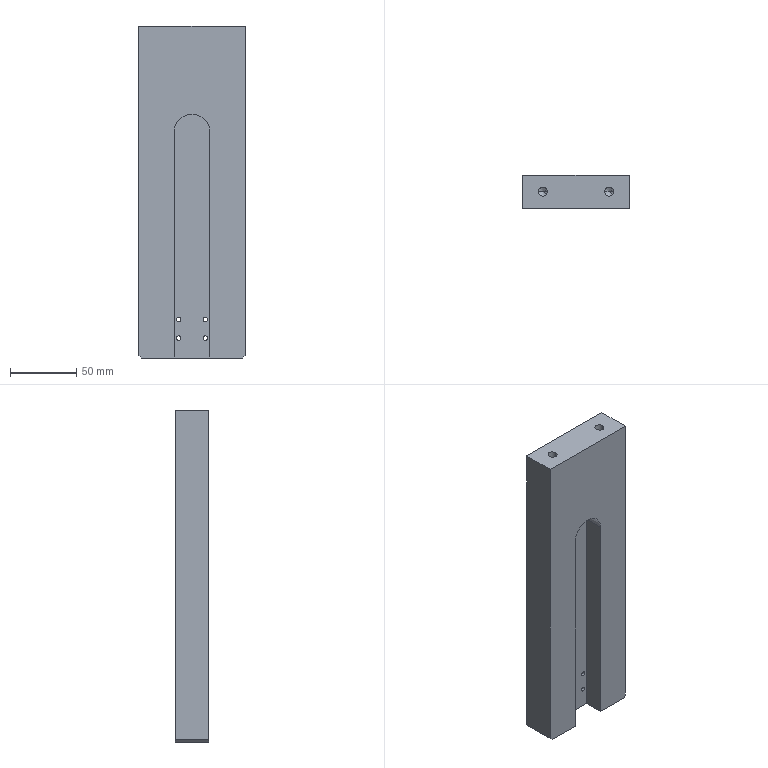Part | SolidWorks | features HoleWzd 5, ICE 2, MirrorPattern 2, Chamfer 1, Extrusion 1 | 1 solid | 28 faces | box 80 x 25 x 250 mm | volume 424930 mm3 | cylinder 13 | plane 11 | cone 4 | commonest cylinder face diameters 3.3 x8 6.8 x4 27 x1
STEP:
#1=CARTESIAN_POINT('',(-28.4,0.,-19.75));
#2=VERTEX_POINT('',#1);
#3=CARTESIAN_POINT('',(-21.6,0.,-19.75));
#4=VERTEX_POINT('',#3);
#5=CARTESIAN_POINT('',(-25.,0.,-19.75));
#6=DIRECTION('',(0.,0.,1.));
#7=DIRECTION('',(1.,0.,0.));
#8=AXIS2_PLACEMENT_3D('',#5,#6,#7);
#9=CIRCLE('',#8,3.4);
#10=EDGE_CURVE('',#2,#4,#9,.T.);
#11=ORIENTED_EDGE('',*,*,#10,.F.);
#12=CARTESIAN_POINT('',(-28.4,0.,0.));
#13=VERTEX_POINT('',#12);
#14=CARTESIAN_POINT('',(-28.4,0.,0.));
#15=DIRECTION('',(0.,0.,1.));
#16=VECTOR('',#15,1000.);
#17=LINE('',#14,#16);
#18=EDGE_CURVE('',#2,#13,#17,.T.);
#19=ORIENTED_EDGE('',*,*,#18,.T.);
#20=CARTESIAN_POINT('',(-21.6,0.,0.));
#21=VERTEX_POINT('',#20);
#22=CARTESIAN_POINT('',(-25.,0.,0.));
#23=DIRECTION('',(0.,0.,1.));
#24=DIRECTION('',(1.,0.,0.));
#25=AXIS2_PLACEMENT_3D('',#22,#23,#24);
#26=CIRCLE('',#25,3.4);
#27=EDGE_CURVE('',#13,#21,#26,.T.);
#28=ORIENTED_EDGE('',*,*,#27,.T.);
#29=CARTESIAN_POINT('',(-21.6,0.,0.));
#30=DIRECTION('',(0.,0.,1.));
#31=VECTOR('',#30,1000.);
#32=LINE('',#29,#31);
#33=EDGE_CURVE('',#4,#21,#32,.T.);
#34=ORIENTED_EDGE('',*,*,#33,.F.);
#35=EDGE_LOOP('',(#11,#19,#28,#34));
#36=FACE_OUTER_BOUND('',#35,.T.);
#37=CARTESIAN_POINT('',(-25.,0.,0.));
#38=DIRECTION('',(0.,0.,1.));
#39=DIRECTION('',(1.,0.,0.));
#40=AXIS2_PLACEMENT_3D('',#37,#38,#39);
#41=CYLINDRICAL_SURFACE('',#40,3.4);
#42=ADVANCED_FACE('',(#36),#41,.F.);
#43=CARTESIAN_POINT('',(-25.,0.,-21.793));
#44=VERTEX_POINT('',#43);
#45=CARTESIAN_POINT('',(-21.6,0.,-19.75));
#46=DIRECTION('',(0.8572,0.,0.515));
#47=VECTOR('',#46,1000.);
#48=LINE('',#45,#47);
#49=EDGE_CURVE('',#44,#4,#48,.T.);
#50=ORIENTED_EDGE('',*,*,#49,.F.);
#51=CARTESIAN_POINT('',(-28.4,0.,-19.75));
#52=DIRECTION('',(-0.8572,0.,0.515));
#53=VECTOR('',#52,1000.);
#54=LINE('',#51,#53);
#55=EDGE_CURVE('',#44,#2,#54,.T.);
#56=ORIENTED_EDGE('',*,*,#55,.T.);
#57=ORIENTED_EDGE('',*,*,#10,.T.);
#58=EDGE_LOOP('',(#50,#56,#57));
#59=FACE_OUTER_BOUND('',#58,.T.);
#60=CARTESIAN_POINT('',(-25.,0.,-19.75));
#61=DIRECTION('',(0.,0.,1.));
#62=DIRECTION('',(1.,0.,0.));
#63=AXIS2_PLACEMENT_3D('',#60,#61,#62);
#64=CONICAL_SURFACE('',#63,3.4,1.03);
#65=ADVANCED_FACE('',(#59),#64,.F.);
#66=CARTESIAN_POINT('',(21.6,0.,-19.75));
#67=VERTEX_POINT('',#66);
#68=CARTESIAN_POINT('',(28.4,0.,-19.75));
#69=VERTEX_POINT('',#68);
#70=CARTESIAN_POINT('',(25.,0.,-19.75));
#71=DIRECTION('',(0.,0.,1.));
#72=DIRECTION('',(1.,0.,0.));
#73=AXIS2_PLACEMENT_3D('',#70,#71,#72);
#74=CIRCLE('',#73,3.4);
#75=EDGE_CURVE('',#67,#69,#74,.T.);
#76=ORIENTED_EDGE('',*,*,#75,.F.);
#77=CARTESIAN_POINT('',(21.6,0.,0.));
#78=VERTEX_POINT('',#77);
#79=CARTESIAN_POINT('',(21.6,0.,0.));
#80=DIRECTION('',(0.,0.,1.));
#81=VECTOR('',#80,1000.);
#82=LINE('',#79,#81);
#83=EDGE_CURVE('',#67,#78,#82,.T.);
#84=ORIENTED_EDGE('',*,*,#83,.T.);
#85=CARTESIAN_POINT('',(28.4,0.,0.));
#86=VERTEX_POINT('',#85);
#87=CARTESIAN_POINT('',(25.,0.,0.));
#88=DIRECTION('',(0.,0.,1.));
#89=DIRECTION('',(1.,0.,0.));
#90=AXIS2_PLACEMENT_3D('',#87,#88,#89);
#91=CIRCLE('',#90,3.4);
#92=EDGE_CURVE('',#78,#86,#91,.T.);
#93=ORIENTED_EDGE('',*,*,#92,.T.);
#94=CARTESIAN_POINT('',(28.4,0.,0.));
#95=DIRECTION('',(0.,0.,1.));
#96=VECTOR('',#95,1000.);
#97=LINE('',#94,#96);
#98=EDGE_CURVE('',#69,#86,#97,.T.);
#99=ORIENTED_EDGE('',*,*,#98,.F.);
#100=EDGE_LOOP('',(#76,#84,#93,#99));
#101=FACE_OUTER_BOUND('',#100,.T.);
#102=CARTESIAN_POINT('',(25.,0.,0.));
#103=DIRECTION('',(0.,0.,1.));
#104=DIRECTION('',(1.,0.,0.));
#105=AXIS2_PLACEMENT_3D('',#102,#103,#104);
#106=CYLINDRICAL_SURFACE('',#105,3.4);
#107=ADVANCED_FACE('',(#101),#106,.F.);
#108=CARTESIAN_POINT('',(25.,0.,-21.793));
#109=VERTEX_POINT('',#108);
#110=CARTESIAN_POINT('',(28.4,0.,-19.75));
#111=DIRECTION('',(0.8572,0.,0.515));
#112=VECTOR('',#111,1000.);
#113=LINE('',#110,#112);
#114=EDGE_CURVE('',#109,#69,#113,.T.);
#115=ORIENTED_EDGE('',*,*,#114,.F.);
#116=CARTESIAN_POINT('',(21.6,0.,-19.75));
#117=DIRECTION('',(-0.8572,0.,0.515));
#118=VECTOR('',#117,1000.);
#119=LINE('',#116,#118);
#120=EDGE_CURVE('',#109,#67,#119,.T.);
#121=ORIENTED_EDGE('',*,*,#120,.T.);
#122=ORIENTED_EDGE('',*,*,#75,.T.);
#123=EDGE_LOOP('',(#115,#121,#122));
#124=FACE_OUTER_BOUND('',#123,.T.);
#125=CARTESIAN_POINT('',(25.,0.,-19.75));
#126=DIRECTION('',(0.,0.,1.));
#127=DIRECTION('',(1.,0.,0.));
#128=AXIS2_PLACEMENT_3D('',#125,#126,#127);
#129=CONICAL_SURFACE('',#128,3.4,1.03);
#130=ADVANCED_FACE('',(#124),#129,.F.);
#131=CARTESIAN_POINT('',(-10.,2.5,-233.35));
#132=VERTEX_POINT('',#131);
#133=CARTESIAN_POINT('',(-10.,2.5,-236.65));
#134=VERTEX_POINT('',#133);
#135=CARTESIAN_POINT('',(-10.,2.5,-235.));
#136=DIRECTION('',(0.,-1.,0.));
#137=DIRECTION('',(0.,0.,-1.));
#138=AXIS2_PLACEMENT_3D('',#135,#136,#137);
#139=CIRCLE('',#138,1.65);
#140=EDGE_CURVE('',#132,#134,#139,.T.);
#141=ORIENTED_EDGE('',*,*,#140,.T.);
#142=CARTESIAN_POINT('',(-10.,12.5,-236.65));
#143=VERTEX_POINT('',#142);
#144=CARTESIAN_POINT('',(-10.,12.5,-236.65));
#145=DIRECTION('',(0.,1.,0.));
#146=VECTOR('',#145,1000.);
#147=LINE('',#144,#146);
#148=EDGE_CURVE('',#134,#143,#147,.T.);
#149=ORIENTED_EDGE('',*,*,#148,.T.);
#150=CARTESIAN_POINT('',(-10.,12.5,-233.35));
#151=VERTEX_POINT('',#150);
#152=CARTESIAN_POINT('',(-10.,12.5,-235.));
#153=DIRECTION('',(0.,1.,0.));
#154=DIRECTION('',(0.,0.,1.));
#155=AXIS2_PLACEMENT_3D('',#152,#153,#154);
#156=CIRCLE('',#155,1.65);
#157=EDGE_CURVE('',#143,#151,#156,.T.);
#158=ORIENTED_EDGE('',*,*,#157,.T.);
#159=CARTESIAN_POINT('',(-10.,12.5,-233.35));
#160=DIRECTION('',(0.,1.,0.));
#161=VECTOR('',#160,1000.);
#162=LINE('',#159,#161);
#163=EDGE_CURVE('',#132,#151,#162,.T.);
#164=ORIENTED_EDGE('',*,*,#163,.F.);
#165=EDGE_LOOP('',(#141,#149,#158,#164));
#166=FACE_OUTER_BOUND('',#165,.T.);
#167=CARTESIAN_POINT('',(-10.,12.5,-235.));
#168=DIRECTION('',(0.,1.,0.));
#169=DIRECTION('',(0.,0.,1.));
#170=AXIS2_PLACEMENT_3D('',#167,#168,#169);
#171=CYLINDRICAL_SURFACE('',#170,1.65);
#172=ADVANCED_FACE('',(#166),#171,.F.);
#173=CARTESIAN_POINT('',(-10.,2.5,-219.35));
#174=VERTEX_POINT('',#173);
#175=CARTESIAN_POINT('',(-10.,2.5,-222.65));
#176=VERTEX_POINT('',#175);
#177=CARTESIAN_POINT('',(-10.,2.5,-221.));
#178=DIRECTION('',(0.,-1.,0.));
#179=DIRECTION('',(0.,0.,-1.));
#180=AXIS2_PLACEMENT_3D('',#177,#178,#179);
#181=CIRCLE('',#180,1.65);
#182=EDGE_CURVE('',#174,#176,#181,.T.);
#183=ORIENTED_EDGE('',*,*,#182,.T.);
#184=CARTESIAN_POINT('',(-10.,12.5,-222.65));
#185=VERTEX_POINT('',#184);
#186=CARTESIAN_POINT('',(-10.,12.5,-222.65));
#187=DIRECTION('',(0.,1.,0.));
#188=VECTOR('',#187,1000.);
#189=LINE('',#186,#188);
#190=EDGE_CURVE('',#176,#185,#189,.T.);
#191=ORIENTED_EDGE('',*,*,#190,.T.);
#192=CARTESIAN_POINT('',(-10.,12.5,-219.35));
#193=VERTEX_POINT('',#192);
#194=CARTESIAN_POINT('',(-10.,12.5,-221.));
#195=DIRECTION('',(0.,1.,0.));
#196=DIRECTION('',(0.,0.,1.));
#197=AXIS2_PLACEMENT_3D('',#194,#195,#196);
#198=CIRCLE('',#197,1.65);
#199=EDGE_CURVE('',#185,#193,#198,.T.);
#200=ORIENTED_EDGE('',*,*,#199,.T.);
#201=CARTESIAN_POINT('',(-10.,12.5,-219.35));
#202=DIRECTION('',(0.,1.,0.));
#203=VECTOR('',#202,1000.);
#204=LINE('',#201,#203);
#205=EDGE_CURVE('',#174,#193,#204,.T.);
#206=ORIENTED_EDGE('',*,*,#205,.F.);
#207=EDGE_LOOP('',(#183,#191,#200,#206));
#208=FACE_OUTER_BOUND('',#207,.T.);
#209=CARTESIAN_POINT('',(-10.,12.5,-221.));
#210=DIRECTION('',(0.,1.,0.));
#211=DIRECTION('',(0.,0.,1.));
#212=AXIS2_PLACEMENT_3D('',#209,#210,#211);
#213=CYLINDRICAL_SURFACE('',#212,1.65);
#214=ADVANCED_FACE('',(#208),#213,.F.);
#215=CARTESIAN_POINT('',(10.,2.5,-219.35));
#216=VERTEX_POINT('',#215);
#217=CARTESIAN_POINT('',(10.,2.5,-222.65));
#218=VERTEX_POINT('',#217);
#219=CARTESIAN_POINT('',(10.,2.5,-221.));
#220=DIRECTION('',(0.,-1.,0.));
#221=DIRECTION('',(0.,0.,-1.));
#222=AXIS2_PLACEMENT_3D('',#219,#220,#221);
#223=CIRCLE('',#222,1.65);
#224=EDGE_CURVE('',#216,#218,#223,.T.);
#225=ORIENTED_EDGE('',*,*,#224,.T.);
#226=CARTESIAN_POINT('',(10.,12.5,-222.65));
#227=VERTEX_POINT('',#226);
#228=CARTESIAN_POINT('',(10.,12.5,-222.65));
#229=DIRECTION('',(0.,1.,0.));
#230=VECTOR('',#229,1000.);
#231=LINE('',#228,#230);
#232=EDGE_CURVE('',#218,#227,#231,.T.);
#233=ORIENTED_EDGE('',*,*,#232,.T.);
#234=CARTESIAN_POINT('',(10.,12.5,-219.35));
#235=VERTEX_POINT('',#234);
#236=CARTESIAN_POINT('',(10.,12.5,-221.));
#237=DIRECTION('',(0.,1.,0.));
#238=DIRECTION('',(0.,0.,1.));
#239=AXIS2_PLACEMENT_3D('',#236,#237,#238);
#240=CIRCLE('',#239,1.65);
#241=EDGE_CURVE('',#227,#235,#240,.T.);
#242=ORIENTED_EDGE('',*,*,#241,.T.);
#243=CARTESIAN_POINT('',(10.,12.5,-219.35));
#244=DIRECTION('',(0.,1.,0.));
#245=VECTOR('',#244,1000.);
#246=LINE('',#243,#245);
#247=EDGE_CURVE('',#216,#235,#246,.T.);
#248=ORIENTED_EDGE('',*,*,#247,.F.);
#249=EDGE_LOOP('',(#225,#233,#242,#248));
#250=FACE_OUTER_BOUND('',#249,.T.);
#251=CARTESIAN_POINT('',(10.,12.5,-221.));
#252=DIRECTION('',(0.,1.,0.));
#253=DIRECTION('',(0.,0.,1.));
#254=AXIS2_PLACEMENT_3D('',#251,#252,#253);
#255=CYLINDRICAL_SURFACE('',#254,1.65);
#256=ADVANCED_FACE('',(#250),#255,.F.);
#257=CARTESIAN_POINT('',(10.,2.5,-233.35));
#258=VERTEX_POINT('',#257);
#259=CARTESIAN_POINT('',(10.,2.5,-236.65));
#260=VERTEX_POINT('',#259);
#261=CARTESIAN_POINT('',(10.,2.5,-235.));
#262=DIRECTION('',(0.,-1.,0.));
#263=DIRECTION('',(0.,0.,-1.));
#264=AXIS2_PLACEMENT_3D('',#261,#262,#263);
#265=CIRCLE('',#264,1.65);
#266=EDGE_CURVE('',#258,#260,#265,.T.);
#267=ORIENTED_EDGE('',*,*,#266,.T.);
#268=CARTESIAN_POINT('',(10.,12.5,-236.65));
#269=VERTEX_POINT('',#268);
#270=CARTESIAN_POINT('',(10.,12.5,-236.65));
#271=DIRECTION('',(0.,1.,0.));
#272=VECTOR('',#271,1000.);
#273=LINE('',#270,#272);
#274=EDGE_CURVE('',#260,#269,#273,.T.);
#275=ORIENTED_EDGE('',*,*,#274,.T.);
#276=CARTESIAN_POINT('',(10.,12.5,-233.35));
#277=VERTEX_POINT('',#276);
#278=CARTESIAN_POINT('',(10.,12.5,-235.));
#279=DIRECTION('',(0.,1.,0.));
#280=DIRECTION('',(0.,0.,1.));
#281=AXIS2_PLACEMENT_3D('',#278,#279,#280);
#282=CIRCLE('',#281,1.65);
#283=EDGE_CURVE('',#269,#277,#282,.T.);
#284=ORIENTED_EDGE('',*,*,#283,.T.);
#285=CARTESIAN_POINT('',(10.,12.5,-233.35));
#286=DIRECTION('',(0.,1.,0.));
#287=VECTOR('',#286,1000.);
#288=LINE('',#285,#287);
#289=EDGE_CURVE('',#258,#277,#288,.T.);
#290=ORIENTED_EDGE('',*,*,#289,.F.);
#291=EDGE_LOOP('',(#267,#275,#284,#290));
#292=FACE_OUTER_BOUND('',#291,.T.);
#293=CARTESIAN_POINT('',(10.,12.5,-235.));
#294=DIRECTION('',(0.,1.,0.));
#295=DIRECTION('',(0.,0.,1.));
#296=AXIS2_PLACEMENT_3D('',#293,#294,#295);
#297=CYLINDRICAL_SURFACE('',#296,1.65);
#298=ADVANCED_FACE('',(#292),#297,.F.);
#299=CARTESIAN_POINT('',(-25.,0.,0.));
#300=DIRECTION('',(0.,0.,1.));
#301=DIRECTION('',(1.,0.,0.));
#302=AXIS2_PLACEMENT_3D('',#299,#300,#301);
#303=CIRCLE('',#302,3.4);
#304=EDGE_CURVE('',#21,#13,#303,.T.);
#305=ORIENTED_EDGE('',*,*,#304,.F.);
#306=ORIENTED_EDGE('',*,*,#27,.F.);
#307=EDGE_LOOP('',(#305,#306));
#308=FACE_BOUND('',#307,.T.);
#309=CARTESIAN_POINT('',(25.,0.,0.));
#310=DIRECTION('',(0.,0.,1.));
#311=DIRECTION('',(1.,0.,0.));
#312=AXIS2_PLACEMENT_3D('',#309,#310,#311);
#313=CIRCLE('',#312,3.4);
#314=EDGE_CURVE('',#86,#78,#313,.T.);
#315=ORIENTED_EDGE('',*,*,#314,.F.);
#316=ORIENTED_EDGE('',*,*,#92,.F.);
#317=EDGE_LOOP('',(#315,#316));
#318=FACE_BOUND('',#317,.T.);
#319=CARTESIAN_POINT('',(-40.,-12.5,0.));
#320=VERTEX_POINT('',#319);
#321=CARTESIAN_POINT('',(40.,-12.5,0.));
#322=VERTEX_POINT('',#321);
#323=CARTESIAN_POINT('',(-75.,-12.5,0.));
#324=DIRECTION('',(1.,0.,0.));
#325=VECTOR('',#324,1000.);
#326=LINE('',#323,#325);
#327=EDGE_CURVE('',#320,#322,#326,.T.);
#328=ORIENTED_EDGE('',*,*,#327,.T.);
#329=CARTESIAN_POINT('',(40.,12.5,0.));
#330=VERTEX_POINT('',#329);
#331=CARTESIAN_POINT('',(40.,12.5,0.));
#332=DIRECTION('',(0.,1.,0.));
#333=VECTOR('',#332,1000.);
#334=LINE('',#331,#333);
#335=EDGE_CURVE('',#322,#330,#334,.T.);
#336=ORIENTED_EDGE('',*,*,#335,.T.);
#337=CARTESIAN_POINT('',(-40.,12.5,0.));
#338=VERTEX_POINT('',#337);
#339=CARTESIAN_POINT('',(-75.,12.5,0.));
#340=DIRECTION('',(1.,0.,0.));
#341=VECTOR('',#340,1000.);
#342=LINE('',#339,#341);
#343=EDGE_CURVE('',#338,#330,#342,.T.);
#344=ORIENTED_EDGE('',*,*,#343,.F.);
#345=CARTESIAN_POINT('',(-40.,12.5,0.));
#346=DIRECTION('',(0.,-1.,0.));
#347=VECTOR('',#346,1000.);
#348=LINE('',#345,#347);
#349=EDGE_CURVE('',#338,#320,#348,.T.);
#350=ORIENTED_EDGE('',*,*,#349,.T.);
#351=EDGE_LOOP('',(#328,#336,#344,#350));
#352=FACE_OUTER_BOUND('',#351,.T.);
#353=CARTESIAN_POINT('',(-75.,12.5,0.));
#354=DIRECTION('',(0.,0.,-1.));
#355=DIRECTION('',(-1.,0.,0.));
#356=AXIS2_PLACEMENT_3D('',#353,#354,#355);
#357=PLANE('',#356);
#358=ADVANCED_FACE('',(#308,#318,#352),#357,.F.);
#359=CARTESIAN_POINT('',(40.,-12.5,-248.));
#360=VERTEX_POINT('',#359);
#361=CARTESIAN_POINT('',(40.,-12.5,-12.));
#362=DIRECTION('',(0.,0.,-1.));
#363=VECTOR('',#362,1000.);
#364=LINE('',#361,#363);
#365=EDGE_CURVE('',#322,#360,#364,.T.);
#366=ORIENTED_EDGE('',*,*,#365,.T.);
#367=CARTESIAN_POINT('',(40.,12.5,-248.));
#368=VERTEX_POINT('',#367);
#369=CARTESIAN_POINT('',(40.,12.5,-248.));
#370=DIRECTION('',(0.,1.,0.));
#371=VECTOR('',#370,1000.);
#372=LINE('',#369,#371);
#373=EDGE_CURVE('',#360,#368,#372,.T.);
#374=ORIENTED_EDGE('',*,*,#373,.T.);
#375=CARTESIAN_POINT('',(40.,12.5,-12.));
#376=DIRECTION('',(0.,0.,-1.));
#377=VECTOR('',#376,1000.);
#378=LINE('',#375,#377);
#379=EDGE_CURVE('',#330,#368,#378,.T.);
#380=ORIENTED_EDGE('',*,*,#379,.F.);
#381=ORIENTED_EDGE('',*,*,#335,.F.);
#382=EDGE_LOOP('',(#366,#374,#380,#381));
#383=FACE_OUTER_BOUND('',#382,.T.);
#384=CARTESIAN_POINT('',(40.,12.5,-12.));
#385=DIRECTION('',(-1.,0.,0.));
#386=DIRECTION('',(0.,0.,1.));
#387=AXIS2_PLACEMENT_3D('',#384,#385,#386);
#388=PLANE('',#387);
#389=ADVANCED_FACE('',(#383),#388,.F.);
#390=CARTESIAN_POINT('',(38.,-12.5,-250.));
#391=VERTEX_POINT('',#390);
#392=CARTESIAN_POINT('',(13.5,-12.5,-250.));
#393=VERTEX_POINT('',#392);
#394=CARTESIAN_POINT('',(40.,-12.5,-250.));
#395=DIRECTION('',(-1.,0.,0.));
#396=VECTOR('',#395,1000.);
#397=LINE('',#394,#396);
#398=EDGE_CURVE('',#391,#393,#397,.T.);
#399=ORIENTED_EDGE('',*,*,#398,.T.);
#400=CARTESIAN_POINT('',(13.5,2.5,-250.));
#401=VERTEX_POINT('',#400);
#402=CARTESIAN_POINT('',(13.5,2.5,-250.));
#403=DIRECTION('',(0.,-1.,0.));
#404=VECTOR('',#403,1000.);
#405=LINE('',#402,#404);
#406=EDGE_CURVE('',#401,#393,#405,.T.);
#407=ORIENTED_EDGE('',*,*,#406,.F.);
#408=CARTESIAN_POINT('',(-13.5,2.5,-250.));
#409=VERTEX_POINT('',#408);
#410=CARTESIAN_POINT('',(40.,2.5,-250.));
#411=DIRECTION('',(1.,0.,0.));
#412=VECTOR('',#411,1000.);
#413=LINE('',#410,#412);
#414=EDGE_CURVE('',#409,#401,#413,.T.);
#415=ORIENTED_EDGE('',*,*,#414,.F.);
#416=CARTESIAN_POINT('',(-13.5,-12.5,-250.));
#417=VERTEX_POINT('',#416);
#418=CARTESIAN_POINT('',(-13.5,2.5,-250.));
#419=DIRECTION('',(0.,-1.,0.));
#420=VECTOR('',#419,1000.);
#421=LINE('',#418,#420);
#422=EDGE_CURVE('',#409,#417,#421,.T.);
#423=ORIENTED_EDGE('',*,*,#422,.T.);
#424=CARTESIAN_POINT('',(-38.,-12.5,-250.));
#425=VERTEX_POINT('',#424);
#426=CARTESIAN_POINT('',(40.,-12.5,-250.));
#427=DIRECTION('',(-1.,0.,0.));
#428=VECTOR('',#427,1000.);
#429=LINE('',#426,#428);
#430=EDGE_CURVE('',#417,#425,#429,.T.);
#431=ORIENTED_EDGE('',*,*,#430,.T.);
#432=CARTESIAN_POINT('',(-38.,12.5,-250.));
#433=VERTEX_POINT('',#432);
#434=CARTESIAN_POINT('',(-38.,12.5,-250.));
#435=DIRECTION('',(0.,1.,0.));
#436=VECTOR('',#435,1000.);
#437=LINE('',#434,#436);
#438=EDGE_CURVE('',#425,#433,#437,.T.);
#439=ORIENTED_EDGE('',*,*,#438,.T.);
#440=CARTESIAN_POINT('',(38.,12.5,-250.));
#441=VERTEX_POINT('',#440);
#442=CARTESIAN_POINT('',(40.,12.5,-250.));
#443=DIRECTION('',(-1.,0.,0.));
#444=VECTOR('',#443,1000.);
#445=LINE('',#442,#444);
#446=EDGE_CURVE('',#441,#433,#445,.T.);
#447=ORIENTED_EDGE('',*,*,#446,.F.);
#448=CARTESIAN_POINT('',(38.,12.5,-250.));
#449=DIRECTION('',(0.,-1.,0.));
#450=VECTOR('',#449,1000.);
#451=LINE('',#448,#450);
#452=EDGE_CURVE('',#441,#391,#451,.T.);
#453=ORIENTED_EDGE('',*,*,#452,.T.);
#454=EDGE_LOOP('',(#399,#407,#415,#423,#431,#439,#447,#453));
#455=FACE_OUTER_BOUND('',#454,.T.);
#456=CARTESIAN_POINT('',(40.,12.5,-250.));
#457=DIRECTION('',(0.,0.,1.));
#458=DIRECTION('',(1.,0.,0.));
#459=AXIS2_PLACEMENT_3D('',#456,#457,#458);
#460=PLANE('',#459);
#461=ADVANCED_FACE('',(#455),#460,.F.);
#462=CARTESIAN_POINT('',(-40.,12.5,-248.));
#463=VERTEX_POINT('',#462);
#464=CARTESIAN_POINT('',(-40.,12.5,-250.));
#465=DIRECTION('',(0.,0.,1.));
#466=VECTOR('',#465,1000.);
#467=LINE('',#464,#466);
#468=EDGE_CURVE('',#463,#338,#467,.T.);
#469=ORIENTED_EDGE('',*,*,#468,.F.);
#470=CARTESIAN_POINT('',(-40.,-12.5,-248.));
#471=VERTEX_POINT('',#470);
#472=CARTESIAN_POINT('',(-40.,12.5,-248.));
#473=DIRECTION('',(0.,-1.,0.));
#474=VECTOR('',#473,1000.);
#475=LINE('',#472,#474);
#476=EDGE_CURVE('',#463,#471,#475,.T.);
#477=ORIENTED_EDGE('',*,*,#476,.T.);
#478=CARTESIAN_POINT('',(-40.,-12.5,-250.));
#479=DIRECTION('',(0.,0.,1.));
#480=VECTOR('',#479,1000.);
#481=LINE('',#478,#480);
#482=EDGE_CURVE('',#471,#320,#481,.T.);
#483=ORIENTED_EDGE('',*,*,#482,.T.);
#484=ORIENTED_EDGE('',*,*,#349,.F.);
#485=EDGE_LOOP('',(#469,#477,#483,#484));
#486=FACE_OUTER_BOUND('',#485,.T.);
#487=CARTESIAN_POINT('',(-40.,12.5,-250.));
#488=DIRECTION('',(1.,0.,0.));
#489=DIRECTION('',(0.,0.,-1.));
#490=AXIS2_PLACEMENT_3D('',#487,#488,#489);
#491=PLANE('',#490);
#492=ADVANCED_FACE('',(#486),#491,.F.);
#493=ORIENTED_EDGE('',*,*,#343,.T.);
#494=ORIENTED_EDGE('',*,*,#379,.T.);
#495=CARTESIAN_POINT('',(144.,12.5,-144.));
#496=DIRECTION('',(-0.7071,0.,-0.7071));
#497=VECTOR('',#496,1000.);
#498=LINE('',#495,#497);
#499=EDGE_CURVE('',#368,#441,#498,.T.);
#500=ORIENTED_EDGE('',*,*,#499,.T.);
#501=ORIENTED_EDGE('',*,*,#446,.T.);
#502=CARTESIAN_POINT('',(-144.,12.5,-144.));
#503=DIRECTION('',(-0.7071,0.,0.7071));
#504=VECTOR('',#503,1000.);
#505=LINE('',#502,#504);
#506=EDGE_CURVE('',#433,#463,#505,.T.);
#507=ORIENTED_EDGE('',*,*,#506,.T.);
#508=ORIENTED_EDGE('',*,*,#468,.T.);
#509=EDGE_LOOP('',(#493,#494,#500,#501,#507,#508));
#510=FACE_OUTER_BOUND('',#509,.T.);
#511=CARTESIAN_POINT('',(-10.,12.5,-235.));
#512=DIRECTION('',(0.,1.,0.));
#513=DIRECTION('',(0.,0.,1.));
#514=AXIS2_PLACEMENT_3D('',#511,#512,#513);
#515=CIRCLE('',#514,1.65);
#516=EDGE_CURVE('',#151,#143,#515,.T.);
#517=ORIENTED_EDGE('',*,*,#516,.F.);
#518=ORIENTED_EDGE('',*,*,#157,.F.);
#519=EDGE_LOOP('',(#517,#518));
#520=FACE_BOUND('',#519,.T.);
#521=CARTESIAN_POINT('',(-10.,12.5,-221.));
#522=DIRECTION('',(0.,1.,0.));
#523=DIRECTION('',(0.,0.,1.));
#524=AXIS2_PLACEMENT_3D('',#521,#522,#523);
#525=CIRCLE('',#524,1.65);
#526=EDGE_CURVE('',#193,#185,#525,.T.);
#527=ORIENTED_EDGE('',*,*,#526,.F.);
#528=ORIENTED_EDGE('',*,*,#199,.F.);
#529=EDGE_LOOP('',(#527,#528));
#530=FACE_BOUND('',#529,.T.);
#531=CARTESIAN_POINT('',(10.,12.5,-221.));
#532=DIRECTION('',(0.,1.,0.));
#533=DIRECTION('',(0.,0.,1.));
#534=AXIS2_PLACEMENT_3D('',#531,#532,#533);
#535=CIRCLE('',#534,1.65);
#536=EDGE_CURVE('',#235,#227,#535,.T.);
#537=ORIENTED_EDGE('',*,*,#536,.F.);
#538=ORIENTED_EDGE('',*,*,#241,.F.);
#539=EDGE_LOOP('',(#537,#538));
#540=FACE_BOUND('',#539,.T.);
#541=CARTESIAN_POINT('',(10.,12.5,-235.));
#542=DIRECTION('',(0.,1.,0.));
#543=DIRECTION('',(0.,0.,1.));
#544=AXIS2_PLACEMENT_3D('',#541,#542,#543);
#545=CIRCLE('',#544,1.65);
#546=EDGE_CURVE('',#277,#269,#545,.T.);
#547=ORIENTED_EDGE('',*,*,#546,.F.);
#548=ORIENTED_EDGE('',*,*,#283,.F.);
#549=EDGE_LOOP('',(#547,#548));
#550=FACE_BOUND('',#549,.T.);
#551=CARTESIAN_POINT('',(0.,12.5,0.));
#552=DIRECTION('',(0.,1.,0.));
#553=DIRECTION('',(0.,0.,1.));
#554=AXIS2_PLACEMENT_3D('',#551,#552,#553);
#555=PLANE('',#554);
#556=ADVANCED_FACE('',(#510,#520,#530,#540,#550),#555,.T.);
#557=ORIENTED_EDGE('',*,*,#365,.F.);
#558=ORIENTED_EDGE('',*,*,#327,.F.);
#559=ORIENTED_EDGE('',*,*,#482,.F.);
#560=CARTESIAN_POINT('',(-40.,-12.5,-248.));
#561=DIRECTION('',(0.7071,0.,-0.7071));
#562=VECTOR('',#561,1000.);
#563=LINE('',#560,#562);
#564=EDGE_CURVE('',#471,#425,#563,.T.);
#565=ORIENTED_EDGE('',*,*,#564,.T.);
#566=ORIENTED_EDGE('',*,*,#430,.F.);
#567=CARTESIAN_POINT('',(-13.5,-12.5,-80.));
#568=VERTEX_POINT('',#567);
#569=CARTESIAN_POINT('',(-13.5,-12.5,-80.));
#570=DIRECTION('',(0.,0.,-1.));
#571=VECTOR('',#570,1000.);
#572=LINE('',#569,#571);
#573=EDGE_CURVE('',#568,#417,#572,.T.);
#574=ORIENTED_EDGE('',*,*,#573,.F.);
#575=CARTESIAN_POINT('',(13.5,-12.5,-80.));
#576=VERTEX_POINT('',#575);
#577=CARTESIAN_POINT('',(0.,-12.5,-80.));
#578=DIRECTION('',(0.,-1.,0.));
#579=DIRECTION('',(0.,0.,-1.));
#580=AXIS2_PLACEMENT_3D('',#577,#578,#579);
#581=CIRCLE('',#580,13.5);
#582=EDGE_CURVE('',#576,#568,#581,.T.);
#583=ORIENTED_EDGE('',*,*,#582,.F.);
#584=CARTESIAN_POINT('',(13.5,-12.5,-80.));
#585=DIRECTION('',(0.,0.,1.));
#586=VECTOR('',#585,1000.);
#587=LINE('',#584,#586);
#588=EDGE_CURVE('',#393,#576,#587,.T.);
#589=ORIENTED_EDGE('',*,*,#588,.F.);
#590=ORIENTED_EDGE('',*,*,#398,.F.);
#591=CARTESIAN_POINT('',(38.,-12.5,-250.));
#592=DIRECTION('',(0.7071,0.,0.7071));
#593=VECTOR('',#592,1000.);
#594=LINE('',#591,#593);
#595=EDGE_CURVE('',#391,#360,#594,.T.);
#596=ORIENTED_EDGE('',*,*,#595,.T.);
#597=EDGE_LOOP('',(#557,#558,#559,#565,#566,#574,#583,#589,#590,#596));
#598=FACE_OUTER_BOUND('',#597,.T.);
#599=CARTESIAN_POINT('',(0.,-12.5,0.));
#600=DIRECTION('',(0.,1.,0.));
#601=DIRECTION('',(0.,0.,1.));
#602=AXIS2_PLACEMENT_3D('',#599,#600,#601);
#603=PLANE('',#602);
#604=ADVANCED_FACE('',(#598),#603,.F.);
#605=ORIENTED_EDGE('',*,*,#499,.F.);
#606=ORIENTED_EDGE('',*,*,#373,.F.);
#607=ORIENTED_EDGE('',*,*,#595,.F.);
#608=ORIENTED_EDGE('',*,*,#452,.F.);
#609=EDGE_LOOP('',(#605,#606,#607,#608));
#610=FACE_OUTER_BOUND('',#609,.T.);
#611=CARTESIAN_POINT('',(38.,12.5,-250.));
#612=DIRECTION('',(-0.7071,0.,0.7071));
#613=DIRECTION('',(0.,-1.,0.));
#614=AXIS2_PLACEMENT_3D('',#611,#612,#613);
#615=PLANE('',#614);
#616=ADVANCED_FACE('',(#610),#615,.F.);
#617=ORIENTED_EDGE('',*,*,#506,.F.);
#618=ORIENTED_EDGE('',*,*,#438,.F.);
#619=ORIENTED_EDGE('',*,*,#564,.F.);
#620=ORIENTED_EDGE('',*,*,#476,.F.);
#621=EDGE_LOOP('',(#617,#618,#619,#620));
#622=FACE_OUTER_BOUND('',#621,.T.);
#623=CARTESIAN_POINT('',(-40.,12.5,-248.));
#624=DIRECTION('',(0.7071,0.,0.7071));
#625=DIRECTION('',(0.,-1.,0.));
#626=AXIS2_PLACEMENT_3D('',#623,#624,#625);
#627=PLANE('',#626);
#628=ADVANCED_FACE('',(#622),#627,.F.);
#629=ORIENTED_EDGE('',*,*,#140,.F.);
#630=CARTESIAN_POINT('',(-10.,2.5,-235.));
#631=DIRECTION('',(0.,-1.,0.));
#632=DIRECTION('',(0.,0.,-1.));
#633=AXIS2_PLACEMENT_3D('',#630,#631,#632);
#634=CIRCLE('',#633,1.65);
#635=EDGE_CURVE('',#134,#132,#634,.T.);
#636=ORIENTED_EDGE('',*,*,#635,.F.);
#637=EDGE_LOOP('',(#629,#636));
#638=FACE_BOUND('',#637,.T.);
#639=ORIENTED_EDGE('',*,*,#182,.F.);
#640=CARTESIAN_POINT('',(-10.,2.5,-221.));
#641=DIRECTION('',(0.,-1.,0.));
#642=DIRECTION('',(0.,0.,-1.));
#643=AXIS2_PLACEMENT_3D('',#640,#641,#642);
#644=CIRCLE('',#643,1.65);
#645=EDGE_CURVE('',#176,#174,#644,.T.);
#646=ORIENTED_EDGE('',*,*,#645,.F.);
#647=EDGE_LOOP('',(#639,#646));
#648=FACE_BOUND('',#647,.T.);
#649=ORIENTED_EDGE('',*,*,#224,.F.);
#650=CARTESIAN_POINT('',(10.,2.5,-221.));
#651=DIRECTION('',(0.,-1.,0.));
#652=DIRECTION('',(0.,0.,-1.));
#653=AXIS2_PLACEMENT_3D('',#650,#651,#652);
#654=CIRCLE('',#653,1.65);
#655=EDGE_CURVE('',#218,#216,#654,.T.);
#656=ORIENTED_EDGE('',*,*,#655,.F.);
#657=EDGE_LOOP('',(#649,#656));
#658=FACE_BOUND('',#657,.T.);
#659=ORIENTED_EDGE('',*,*,#266,.F.);
#660=CARTESIAN_POINT('',(10.,2.5,-235.));
#661=DIRECTION('',(0.,-1.,0.));
#662=DIRECTION('',(0.,0.,-1.));
#663=AXIS2_PLACEMENT_3D('',#660,#661,#662);
#664=CIRCLE('',#663,1.65);
#665=EDGE_CURVE('',#260,#258,#664,.T.);
#666=ORIENTED_EDGE('',*,*,#665,.F.);
#667=EDGE_LOOP('',(#659,#666));
#668=FACE_BOUND('',#667,.T.);
#669=ORIENTED_EDGE('',*,*,#414,.T.);
#670=CARTESIAN_POINT('',(13.5,2.5,-80.));
#671=VERTEX_POINT('',#670);
#672=CARTESIAN_POINT('',(13.5,2.5,-80.));
#673=DIRECTION('',(0.,0.,1.));
#674=VECTOR('',#673,1000.);
#675=LINE('',#672,#674);
#676=EDGE_CURVE('',#401,#671,#675,.T.);
#677=ORIENTED_EDGE('',*,*,#676,.T.);
#678=CARTESIAN_POINT('',(-13.5,2.5,-80.));
#679=VERTEX_POINT('',#678);
#680=CARTESIAN_POINT('',(0.,2.5,-80.));
#681=DIRECTION('',(0.,-1.,0.));
#682=DIRECTION('',(0.,0.,-1.));
#683=AXIS2_PLACEMENT_3D('',#680,#681,#682);
#684=CIRCLE('',#683,13.5);
#685=EDGE_CURVE('',#671,#679,#684,.T.);
#686=ORIENTED_EDGE('',*,*,#685,.T.);
#687=CARTESIAN_POINT('',(-13.5,2.5,-80.));
#688=DIRECTION('',(0.,0.,-1.));
#689=VECTOR('',#688,1000.);
#690=LINE('',#687,#689);
#691=EDGE_CURVE('',#679,#409,#690,.T.);
#692=ORIENTED_EDGE('',*,*,#691,.T.);
#693=EDGE_LOOP('',(#669,#677,#686,#692));
#694=FACE_OUTER_BOUND('',#693,.T.);
#695=CARTESIAN_POINT('',(0.,2.5,-80.));
#696=DIRECTION('',(0.,-1.,0.));
#697=DIRECTION('',(0.,0.,-1.));
#698=AXIS2_PLACEMENT_3D('',#695,#696,#697);
#699=PLANE('',#698);
#700=ADVANCED_FACE('',(#638,#648,#658,#668,#694),#699,.T.);
#701=ORIENTED_EDGE('',*,*,#582,.T.);
#702=CARTESIAN_POINT('',(-13.5,2.5,-80.));
#703=DIRECTION('',(0.,-1.,0.));
#704=VECTOR('',#703,1000.);
#705=LINE('',#702,#704);
#706=EDGE_CURVE('',#679,#568,#705,.T.);
#707=ORIENTED_EDGE('',*,*,#706,.F.);
#708=ORIENTED_EDGE('',*,*,#685,.F.);
#709=CARTESIAN_POINT('',(13.5,2.5,-80.));
#710=DIRECTION('',(0.,-1.,0.));
#711=VECTOR('',#710,1000.);
#712=LINE('',#709,#711);
#713=EDGE_CURVE('',#671,#576,#712,.T.);
#714=ORIENTED_EDGE('',*,*,#713,.T.);
#715=EDGE_LOOP('',(#701,#707,#708,#714));
#716=FACE_OUTER_BOUND('',#715,.T.);
#717=CARTESIAN_POINT('',(0.,2.5,-80.));
#718=DIRECTION('',(0.,-1.,0.));
#719=DIRECTION('',(0.,0.,-1.));
#720=AXIS2_PLACEMENT_3D('',#717,#718,#719);
#721=CYLINDRICAL_SURFACE('',#720,13.5);
#722=ADVANCED_FACE('',(#716),#721,.F.);
#723=ORIENTED_EDGE('',*,*,#588,.T.);
#724=ORIENTED_EDGE('',*,*,#713,.F.);
#725=ORIENTED_EDGE('',*,*,#676,.F.);
#726=ORIENTED_EDGE('',*,*,#406,.T.);
#727=EDGE_LOOP('',(#723,#724,#725,#726));
#728=FACE_OUTER_BOUND('',#727,.T.);
#729=CARTESIAN_POINT('',(13.5,2.5,-80.));
#730=DIRECTION('',(1.,0.,0.));
#731=DIRECTION('',(0.,0.,-1.));
#732=AXIS2_PLACEMENT_3D('',#729,#730,#731);
#733=PLANE('',#732);
#734=ADVANCED_FACE('',(#728),#733,.F.);
#735=ORIENTED_EDGE('',*,*,#573,.T.);
#736=ORIENTED_EDGE('',*,*,#422,.F.);
#737=ORIENTED_EDGE('',*,*,#691,.F.);
#738=ORIENTED_EDGE('',*,*,#706,.T.);
#739=EDGE_LOOP('',(#735,#736,#737,#738));
#740=FACE_OUTER_BOUND('',#739,.T.);
#741=CARTESIAN_POINT('',(-13.5,2.5,-80.));
#742=DIRECTION('',(-1.,0.,0.));
#743=DIRECTION('',(0.,0.,1.));
#744=AXIS2_PLACEMENT_3D('',#741,#742,#743);
#745=PLANE('',#744);
#746=ADVANCED_FACE('',(#740),#745,.F.);
#747=ORIENTED_EDGE('',*,*,#274,.F.);
#748=ORIENTED_EDGE('',*,*,#665,.T.);
#749=ORIENTED_EDGE('',*,*,#289,.T.);
#750=ORIENTED_EDGE('',*,*,#546,.T.);
#751=EDGE_LOOP('',(#747,#748,#749,#750));
#752=FACE_OUTER_BOUND('',#751,.T.);
#753=CARTESIAN_POINT('',(10.,12.5,-235.));
#754=DIRECTION('',(0.,1.,0.));
#755=DIRECTION('',(0.,0.,1.));
#756=AXIS2_PLACEMENT_3D('',#753,#754,#755);
#757=CYLINDRICAL_SURFACE('',#756,1.65);
#758=ADVANCED_FACE('',(#752),#757,.F.);
#759=ORIENTED_EDGE('',*,*,#232,.F.);
#760=ORIENTED_EDGE('',*,*,#655,.T.);
#761=ORIENTED_EDGE('',*,*,#247,.T.);
#762=ORIENTED_EDGE('',*,*,#536,.T.);
#763=EDGE_LOOP('',(#759,#760,#761,#762));
#764=FACE_OUTER_BOUND('',#763,.T.);
#765=CARTESIAN_POINT('',(10.,12.5,-221.));
#766=DIRECTION('',(0.,1.,0.));
#767=DIRECTION('',(0.,0.,1.));
#768=AXIS2_PLACEMENT_3D('',#765,#766,#767);
#769=CYLINDRICAL_SURFACE('',#768,1.65);
#770=ADVANCED_FACE('',(#764),#769,.F.);
#771=ORIENTED_EDGE('',*,*,#190,.F.);
#772=ORIENTED_EDGE('',*,*,#645,.T.);
#773=ORIENTED_EDGE('',*,*,#205,.T.);
#774=ORIENTED_EDGE('',*,*,#526,.T.);
#775=EDGE_LOOP('',(#771,#772,#773,#774));
#776=FACE_OUTER_BOUND('',#775,.T.);
#777=CARTESIAN_POINT('',(-10.,12.5,-221.));
#778=DIRECTION('',(0.,1.,0.));
#779=DIRECTION('',(0.,0.,1.));
#780=AXIS2_PLACEMENT_3D('',#777,#778,#779);
#781=CYLINDRICAL_SURFACE('',#780,1.65);
#782=ADVANCED_FACE('',(#776),#781,.F.);
#783=ORIENTED_EDGE('',*,*,#148,.F.);
#784=ORIENTED_EDGE('',*,*,#635,.T.);
#785=ORIENTED_EDGE('',*,*,#163,.T.);
#786=ORIENTED_EDGE('',*,*,#516,.T.);
#787=EDGE_LOOP('',(#783,#784,#785,#786));
#788=FACE_OUTER_BOUND('',#787,.T.);
#789=CARTESIAN_POINT('',(-10.,12.5,-235.));
#790=DIRECTION('',(0.,1.,0.));
#791=DIRECTION('',(0.,0.,1.));
#792=AXIS2_PLACEMENT_3D('',#789,#790,#791);
#793=CYLINDRICAL_SURFACE('',#792,1.65);
#794=ADVANCED_FACE('',(#788),#793,.F.);
#795=ORIENTED_EDGE('',*,*,#120,.F.);
#796=ORIENTED_EDGE('',*,*,#114,.T.);
#797=CARTESIAN_POINT('',(25.,0.,-19.75));
#798=DIRECTION('',(0.,0.,1.));
#799=DIRECTION('',(1.,0.,0.));
#800=AXIS2_PLACEMENT_3D('',#797,#798,#799);
#801=CIRCLE('',#800,3.4);
#802=EDGE_CURVE('',#69,#67,#801,.T.);
#803=ORIENTED_EDGE('',*,*,#802,.T.);
#804=EDGE_LOOP('',(#795,#796,#803));
#805=FACE_OUTER_BOUND('',#804,.T.);
#806=CARTESIAN_POINT('',(25.,0.,-19.75));
#807=DIRECTION('',(0.,0.,1.));
#808=DIRECTION('',(1.,0.,0.));
#809=AXIS2_PLACEMENT_3D('',#806,#807,#808);
#810=CONICAL_SURFACE('',#809,3.4,1.03);
#811=ADVANCED_FACE('',(#805),#810,.F.);
#812=ORIENTED_EDGE('',*,*,#83,.F.);
#813=ORIENTED_EDGE('',*,*,#802,.F.);
#814=ORIENTED_EDGE('',*,*,#98,.T.);
#815=ORIENTED_EDGE('',*,*,#314,.T.);
#816=EDGE_LOOP('',(#812,#813,#814,#815));
#817=FACE_OUTER_BOUND('',#816,.T.);
#818=CARTESIAN_POINT('',(25.,0.,0.));
#819=DIRECTION('',(0.,0.,1.));
#820=DIRECTION('',(1.,0.,0.));
#821=AXIS2_PLACEMENT_3D('',#818,#819,#820);
#822=CYLINDRICAL_SURFACE('',#821,3.4);
#823=ADVANCED_FACE('',(#817),#822,.F.);
#824=ORIENTED_EDGE('',*,*,#55,.F.);
#825=ORIENTED_EDGE('',*,*,#49,.T.);
#826=CARTESIAN_POINT('',(-25.,0.,-19.75));
#827=DIRECTION('',(0.,0.,1.));
#828=DIRECTION('',(1.,0.,0.));
#829=AXIS2_PLACEMENT_3D('',#826,#827,#828);
#830=CIRCLE('',#829,3.4);
#831=EDGE_CURVE('',#4,#2,#830,.T.);
#832=ORIENTED_EDGE('',*,*,#831,.T.);
#833=EDGE_LOOP('',(#824,#825,#832));
#834=FACE_OUTER_BOUND('',#833,.T.);
#835=CARTESIAN_POINT('',(-25.,0.,-19.75));
#836=DIRECTION('',(0.,0.,1.));
#837=DIRECTION('',(1.,0.,0.));
#838=AXIS2_PLACEMENT_3D('',#835,#836,#837);
#839=CONICAL_SURFACE('',#838,3.4,1.03);
#840=ADVANCED_FACE('',(#834),#839,.F.);
#841=ORIENTED_EDGE('',*,*,#18,.F.);
#842=ORIENTED_EDGE('',*,*,#831,.F.);
#843=ORIENTED_EDGE('',*,*,#33,.T.);
#844=ORIENTED_EDGE('',*,*,#304,.T.);
#845=EDGE_LOOP('',(#841,#842,#843,#844));
#846=FACE_OUTER_BOUND('',#845,.T.);
#847=CARTESIAN_POINT('',(-25.,0.,0.));
#848=DIRECTION('',(0.,0.,1.));
#849=DIRECTION('',(1.,0.,0.));
#850=AXIS2_PLACEMENT_3D('',#847,#848,#849);
#851=CYLINDRICAL_SURFACE('',#850,3.4);
#852=ADVANCED_FACE('',(#846),#851,.F.);
#853=CLOSED_SHELL('',(#42,#65,#107,#130,#172,#214,#256,#298,#358,#389,#461,#492,#556,#604,#616,#628,#700,#722,#734,#746,#758,#770,#782,#794,#811,#823,#840,#852));
#854=MANIFOLD_SOLID_BREP('',#853);
#855=CARTESIAN_POINT('',(0.,0.,0.));
#856=DIRECTION('',(0.,0.,1.));
#857=DIRECTION('',(1.,0.,0.));
#858=AXIS2_PLACEMENT_3D('',#855,#856,#857);
#859=(LENGTH_UNIT()NAMED_UNIT(*)SI_UNIT(.MILLI.,.METRE.));
#860=UNCERTAINTY_MEASURE_WITH_UNIT(LENGTH_MEASURE(0.00001),#859,'','');
#861=(NAMED_UNIT(*)PLANE_ANGLE_UNIT()SI_UNIT($,.RADIAN.));
#862=(NAMED_UNIT(*)SI_UNIT($,.STERADIAN.)SOLID_ANGLE_UNIT());
#863=(GEOMETRIC_REPRESENTATION_CONTEXT(3)GLOBAL_UNCERTAINTY_ASSIGNED_CONTEXT((#860))GLOBAL_UNIT_ASSIGNED_CONTEXT((#859,#861,#862))REPRESENTATION_CONTEXT('',''));
#864=ADVANCED_BREP_SHAPE_REPRESENTATION('',(#854,#858),#863);